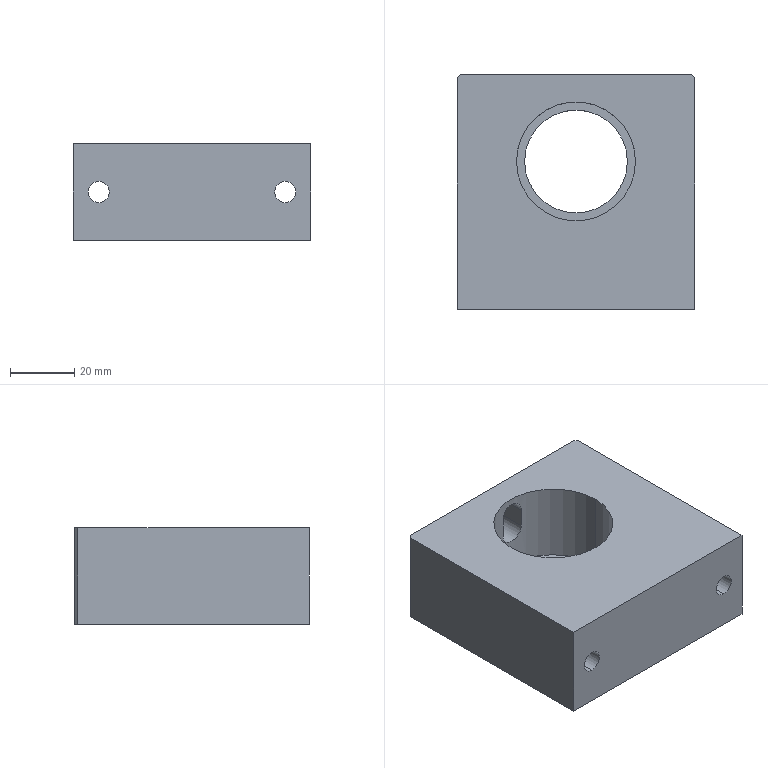Part | SolidWorks | features BaseBody 1 | 1 solid | 28 faces | box 74 x 73 x 30 mm | volume 117987 mm3 | cylinder 15 | plane 13 | commonest cylinder face diameters 6.6 x4 11 x4 8 x3 32 x2 37 x2
STEP:
#1=CARTESIAN_POINT('',(0.,28.,28.));
#2=VERTEX_POINT('',#1);
#3=CARTESIAN_POINT('',(4.,27.562,24.));
#4=VERTEX_POINT('',#3);
#5=CARTESIAN_POINT('',(0.,28.,28.));
#6=CARTESIAN_POINT('',(0.265,28.,28.));
#7=CARTESIAN_POINT('',(0.5253,27.994,27.974));
#8=CARTESIAN_POINT('',(1.037,27.973,27.872));
#9=CARTESIAN_POINT('',(1.292,27.956,27.795));
#10=CARTESIAN_POINT('',(1.776,27.916,27.594));
#11=CARTESIAN_POINT('',(2.005,27.892,27.471));
#12=CARTESIAN_POINT('',(2.439,27.84,27.181));
#13=CARTESIAN_POINT('',(2.644,27.811,27.013));
#14=CARTESIAN_POINT('',(3.012,27.754,26.645));
#15=CARTESIAN_POINT('',(3.177,27.726,26.445));
#16=CARTESIAN_POINT('',(3.469,27.672,26.008));
#17=CARTESIAN_POINT('',(3.593,27.648,25.777));
#18=CARTESIAN_POINT('',(3.793,27.607,25.296));
#19=CARTESIAN_POINT('',(3.87,27.591,25.044));
#20=CARTESIAN_POINT('',(3.974,27.568,24.527));
#21=CARTESIAN_POINT('',(4.,27.562,24.265));
#22=CARTESIAN_POINT('',(4.,27.562,24.));
#23=B_SPLINE_CURVE_WITH_KNOTS('',3,(#5,#6,#7,#8,#9,#10,#11,#12,#13,#14,#15,#16,#17,#18,#19,#20,#21,#22),.UNSPECIFIED.,.F.,.F.,(4,2,2,2,2,2,2,2,4),(0.,0.0007834,0.001567,0.00235,0.003134,0.003917,0.0047,0.005484,0.006267),.UNSPECIFIED.);
#24=EDGE_CURVE('',#2,#4,#23,.T.);
#25=ORIENTED_EDGE('',*,*,#24,.F.);
#26=CARTESIAN_POINT('',(0.,36.5,28.));
#27=VERTEX_POINT('',#26);
#28=CARTESIAN_POINT('',(0.,11.5,28.));
#29=DIRECTION('',(0.,1.,0.));
#30=VECTOR('',#29,1000.);
#31=LINE('',#28,#30);
#32=EDGE_CURVE('',#2,#27,#31,.T.);
#33=ORIENTED_EDGE('',*,*,#32,.T.);
#34=CARTESIAN_POINT('',(4.,36.5,24.));
#35=VERTEX_POINT('',#34);
#36=CARTESIAN_POINT('',(0.,36.5,24.));
#37=DIRECTION('',(0.,1.,0.));
#38=DIRECTION('',(0.,0.,1.));
#39=AXIS2_PLACEMENT_3D('',#36,#37,#38);
#40=CIRCLE('',#39,4.);
#41=EDGE_CURVE('',#27,#35,#40,.T.);
#42=ORIENTED_EDGE('',*,*,#41,.T.);
#43=CARTESIAN_POINT('',(4.,11.5,24.));
#44=DIRECTION('',(0.,1.,0.));
#45=VECTOR('',#44,1000.);
#46=LINE('',#43,#45);
#47=EDGE_CURVE('',#4,#35,#46,.T.);
#48=ORIENTED_EDGE('',*,*,#47,.F.);
#49=EDGE_LOOP('',(#25,#33,#42,#48));
#50=FACE_OUTER_BOUND('',#49,.T.);
#51=CARTESIAN_POINT('',(0.,11.5,24.));
#52=DIRECTION('',(0.,1.,0.));
#53=DIRECTION('',(0.,0.,1.));
#54=AXIS2_PLACEMENT_3D('',#51,#52,#53);
#55=CYLINDRICAL_SURFACE('',#54,4.);
#56=ADVANCED_FACE('',(#50),#55,.F.);
#57=CARTESIAN_POINT('',(-29.,-23.5,9.5));
#58=VERTEX_POINT('',#57);
#59=CARTESIAN_POINT('',(-29.,-23.5,20.5));
#60=VERTEX_POINT('',#59);
#61=CARTESIAN_POINT('',(-29.,-23.5,15.));
#62=DIRECTION('',(0.,1.,0.));
#63=DIRECTION('',(0.,0.,1.));
#64=AXIS2_PLACEMENT_3D('',#61,#62,#63);
#65=CIRCLE('',#64,5.5);
#66=EDGE_CURVE('',#58,#60,#65,.T.);
#67=ORIENTED_EDGE('',*,*,#66,.F.);
#68=CARTESIAN_POINT('',(-29.,36.5,9.5));
#69=VERTEX_POINT('',#68);
#70=CARTESIAN_POINT('',(-29.,36.5,9.5));
#71=DIRECTION('',(0.,1.,0.));
#72=VECTOR('',#71,1000.);
#73=LINE('',#70,#72);
#74=EDGE_CURVE('',#58,#69,#73,.T.);
#75=ORIENTED_EDGE('',*,*,#74,.T.);
#76=CARTESIAN_POINT('',(-29.,36.5,20.5));
#77=VERTEX_POINT('',#76);
#78=CARTESIAN_POINT('',(-29.,36.5,15.));
#79=DIRECTION('',(0.,1.,0.));
#80=DIRECTION('',(0.,0.,1.));
#81=AXIS2_PLACEMENT_3D('',#78,#79,#80);
#82=CIRCLE('',#81,5.5);
#83=EDGE_CURVE('',#69,#77,#82,.T.);
#84=ORIENTED_EDGE('',*,*,#83,.T.);
#85=CARTESIAN_POINT('',(-29.,36.5,20.5));
#86=DIRECTION('',(0.,1.,0.));
#87=VECTOR('',#86,1000.);
#88=LINE('',#85,#87);
#89=EDGE_CURVE('',#60,#77,#88,.T.);
#90=ORIENTED_EDGE('',*,*,#89,.F.);
#91=EDGE_LOOP('',(#67,#75,#84,#90));
#92=FACE_OUTER_BOUND('',#91,.T.);
#93=CARTESIAN_POINT('',(-29.,36.5,15.));
#94=DIRECTION('',(0.,1.,0.));
#95=DIRECTION('',(0.,0.,1.));
#96=AXIS2_PLACEMENT_3D('',#93,#94,#95);
#97=CYLINDRICAL_SURFACE('',#96,5.5);
#98=ADVANCED_FACE('',(#92),#97,.F.);
#99=CARTESIAN_POINT('',(-29.,-36.5,11.7));
#100=VERTEX_POINT('',#99);
#101=CARTESIAN_POINT('',(-29.,-36.5,18.3));
#102=VERTEX_POINT('',#101);
#103=CARTESIAN_POINT('',(-29.,-36.5,15.));
#104=DIRECTION('',(0.,1.,0.));
#105=DIRECTION('',(0.,0.,1.));
#106=AXIS2_PLACEMENT_3D('',#103,#104,#105);
#107=CIRCLE('',#106,3.3);
#108=EDGE_CURVE('',#100,#102,#107,.T.);
#109=ORIENTED_EDGE('',*,*,#108,.F.);
#110=CARTESIAN_POINT('',(-29.,-23.5,11.7));
#111=VERTEX_POINT('',#110);
#112=CARTESIAN_POINT('',(-29.,36.5,11.7));
#113=DIRECTION('',(0.,1.,0.));
#114=VECTOR('',#113,1000.);
#115=LINE('',#112,#114);
#116=EDGE_CURVE('',#100,#111,#115,.T.);
#117=ORIENTED_EDGE('',*,*,#116,.T.);
#118=CARTESIAN_POINT('',(-29.,-23.5,18.3));
#119=VERTEX_POINT('',#118);
#120=CARTESIAN_POINT('',(-29.,-23.5,15.));
#121=DIRECTION('',(0.,1.,0.));
#122=DIRECTION('',(0.,0.,1.));
#123=AXIS2_PLACEMENT_3D('',#120,#121,#122);
#124=CIRCLE('',#123,3.3);
#125=EDGE_CURVE('',#111,#119,#124,.T.);
#126=ORIENTED_EDGE('',*,*,#125,.T.);
#127=CARTESIAN_POINT('',(-29.,36.5,18.3));
#128=DIRECTION('',(0.,1.,0.));
#129=VECTOR('',#128,1000.);
#130=LINE('',#127,#129);
#131=EDGE_CURVE('',#102,#119,#130,.T.);
#132=ORIENTED_EDGE('',*,*,#131,.F.);
#133=EDGE_LOOP('',(#109,#117,#126,#132));
#134=FACE_OUTER_BOUND('',#133,.T.);
#135=CARTESIAN_POINT('',(-29.,36.5,15.));
#136=DIRECTION('',(0.,1.,0.));
#137=DIRECTION('',(0.,0.,1.));
#138=AXIS2_PLACEMENT_3D('',#135,#136,#137);
#139=CYLINDRICAL_SURFACE('',#138,3.3);
#140=ADVANCED_FACE('',(#134),#139,.F.);
#141=CARTESIAN_POINT('',(29.,-23.5,9.5));
#142=VERTEX_POINT('',#141);
#143=CARTESIAN_POINT('',(29.,-23.5,20.5));
#144=VERTEX_POINT('',#143);
#145=CARTESIAN_POINT('',(29.,-23.5,15.));
#146=DIRECTION('',(0.,1.,0.));
#147=DIRECTION('',(0.,0.,1.));
#148=AXIS2_PLACEMENT_3D('',#145,#146,#147);
#149=CIRCLE('',#148,5.5);
#150=EDGE_CURVE('',#142,#144,#149,.T.);
#151=ORIENTED_EDGE('',*,*,#150,.F.);
#152=CARTESIAN_POINT('',(29.,36.5,9.5));
#153=VERTEX_POINT('',#152);
#154=CARTESIAN_POINT('',(29.,36.5,9.5));
#155=DIRECTION('',(0.,1.,0.));
#156=VECTOR('',#155,1000.);
#157=LINE('',#154,#156);
#158=EDGE_CURVE('',#142,#153,#157,.T.);
#159=ORIENTED_EDGE('',*,*,#158,.T.);
#160=CARTESIAN_POINT('',(29.,36.5,20.5));
#161=VERTEX_POINT('',#160);
#162=CARTESIAN_POINT('',(29.,36.5,15.));
#163=DIRECTION('',(0.,1.,0.));
#164=DIRECTION('',(0.,0.,1.));
#165=AXIS2_PLACEMENT_3D('',#162,#163,#164);
#166=CIRCLE('',#165,5.5);
#167=EDGE_CURVE('',#153,#161,#166,.T.);
#168=ORIENTED_EDGE('',*,*,#167,.T.);
#169=CARTESIAN_POINT('',(29.,36.5,20.5));
#170=DIRECTION('',(0.,1.,0.));
#171=VECTOR('',#170,1000.);
#172=LINE('',#169,#171);
#173=EDGE_CURVE('',#144,#161,#172,.T.);
#174=ORIENTED_EDGE('',*,*,#173,.F.);
#175=EDGE_LOOP('',(#151,#159,#168,#174));
#176=FACE_OUTER_BOUND('',#175,.T.);
#177=CARTESIAN_POINT('',(29.,36.5,15.));
#178=DIRECTION('',(0.,1.,0.));
#179=DIRECTION('',(0.,0.,1.));
#180=AXIS2_PLACEMENT_3D('',#177,#178,#179);
#181=CYLINDRICAL_SURFACE('',#180,5.5);
#182=ADVANCED_FACE('',(#176),#181,.F.);
#183=CARTESIAN_POINT('',(29.,-36.5,11.7));
#184=VERTEX_POINT('',#183);
#185=CARTESIAN_POINT('',(29.,-36.5,18.3));
#186=VERTEX_POINT('',#185);
#187=CARTESIAN_POINT('',(29.,-36.5,15.));
#188=DIRECTION('',(0.,1.,0.));
#189=DIRECTION('',(0.,0.,1.));
#190=AXIS2_PLACEMENT_3D('',#187,#188,#189);
#191=CIRCLE('',#190,3.3);
#192=EDGE_CURVE('',#184,#186,#191,.T.);
#193=ORIENTED_EDGE('',*,*,#192,.F.);
#194=CARTESIAN_POINT('',(29.,-23.5,11.7));
#195=VERTEX_POINT('',#194);
#196=CARTESIAN_POINT('',(29.,36.5,11.7));
#197=DIRECTION('',(0.,1.,0.));
#198=VECTOR('',#197,1000.);
#199=LINE('',#196,#198);
#200=EDGE_CURVE('',#184,#195,#199,.T.);
#201=ORIENTED_EDGE('',*,*,#200,.T.);
#202=CARTESIAN_POINT('',(29.,-23.5,18.3));
#203=VERTEX_POINT('',#202);
#204=CARTESIAN_POINT('',(29.,-23.5,15.));
#205=DIRECTION('',(0.,1.,0.));
#206=DIRECTION('',(0.,0.,1.));
#207=AXIS2_PLACEMENT_3D('',#204,#205,#206);
#208=CIRCLE('',#207,3.3);
#209=EDGE_CURVE('',#195,#203,#208,.T.);
#210=ORIENTED_EDGE('',*,*,#209,.T.);
#211=CARTESIAN_POINT('',(29.,36.5,18.3));
#212=DIRECTION('',(0.,1.,0.));
#213=VECTOR('',#212,1000.);
#214=LINE('',#211,#213);
#215=EDGE_CURVE('',#186,#203,#214,.T.);
#216=ORIENTED_EDGE('',*,*,#215,.F.);
#217=EDGE_LOOP('',(#193,#201,#210,#216));
#218=FACE_OUTER_BOUND('',#217,.T.);
#219=CARTESIAN_POINT('',(29.,36.5,15.));
#220=DIRECTION('',(0.,1.,0.));
#221=DIRECTION('',(0.,0.,1.));
#222=AXIS2_PLACEMENT_3D('',#219,#220,#221);
#223=CYLINDRICAL_SURFACE('',#222,3.3);
#224=ADVANCED_FACE('',(#218),#223,.F.);
#225=CARTESIAN_POINT('',(-18.5,9.5,5.));
#226=VERTEX_POINT('',#225);
#227=CARTESIAN_POINT('',(18.5,9.5,5.));
#228=VERTEX_POINT('',#227);
#229=CARTESIAN_POINT('',(0.,9.5,5.));
#230=DIRECTION('',(0.,0.,1.));
#231=DIRECTION('',(1.,0.,0.));
#232=AXIS2_PLACEMENT_3D('',#229,#230,#231);
#233=CIRCLE('',#232,18.5);
#234=EDGE_CURVE('',#226,#228,#233,.T.);
#235=ORIENTED_EDGE('',*,*,#234,.F.);
#236=CARTESIAN_POINT('',(-18.5,9.5,30.));
#237=VERTEX_POINT('',#236);
#238=CARTESIAN_POINT('',(-18.5,9.5,5.));
#239=DIRECTION('',(0.,0.,1.));
#240=VECTOR('',#239,1000.);
#241=LINE('',#238,#240);
#242=EDGE_CURVE('',#226,#237,#241,.T.);
#243=ORIENTED_EDGE('',*,*,#242,.T.);
#244=CARTESIAN_POINT('',(18.5,9.5,30.));
#245=VERTEX_POINT('',#244);
#246=CARTESIAN_POINT('',(0.,9.5,30.));
#247=DIRECTION('',(0.,0.,1.));
#248=DIRECTION('',(1.,0.,0.));
#249=AXIS2_PLACEMENT_3D('',#246,#247,#248);
#250=CIRCLE('',#249,18.5);
#251=EDGE_CURVE('',#237,#245,#250,.T.);
#252=ORIENTED_EDGE('',*,*,#251,.T.);
#253=CARTESIAN_POINT('',(18.5,9.5,5.));
#254=DIRECTION('',(0.,0.,1.));
#255=VECTOR('',#254,1000.);
#256=LINE('',#253,#255);
#257=EDGE_CURVE('',#228,#245,#256,.T.);
#258=ORIENTED_EDGE('',*,*,#257,.F.);
#259=EDGE_LOOP('',(#235,#243,#252,#258));
#260=FACE_OUTER_BOUND('',#259,.T.);
#261=CARTESIAN_POINT('',(0.,9.5,5.));
#262=DIRECTION('',(0.,0.,1.));
#263=DIRECTION('',(1.,0.,0.));
#264=AXIS2_PLACEMENT_3D('',#261,#262,#263);
#265=CYLINDRICAL_SURFACE('',#264,18.5);
#266=ADVANCED_FACE('',(#260),#265,.F.);
#267=CARTESIAN_POINT('',(-16.,9.5,0.));
#268=VERTEX_POINT('',#267);
#269=CARTESIAN_POINT('',(16.,9.5,0.));
#270=VERTEX_POINT('',#269);
#271=CARTESIAN_POINT('',(0.,9.5,0.));
#272=DIRECTION('',(0.,0.,1.));
#273=DIRECTION('',(1.,0.,0.));
#274=AXIS2_PLACEMENT_3D('',#271,#272,#273);
#275=CIRCLE('',#274,16.);
#276=EDGE_CURVE('',#268,#270,#275,.T.);
#277=ORIENTED_EDGE('',*,*,#276,.F.);
#278=CARTESIAN_POINT('',(-16.,9.5,5.));
#279=VERTEX_POINT('',#278);
#280=CARTESIAN_POINT('',(-16.,9.5,0.));
#281=DIRECTION('',(0.,0.,1.));
#282=VECTOR('',#281,1000.);
#283=LINE('',#280,#282);
#284=EDGE_CURVE('',#268,#279,#283,.T.);
#285=ORIENTED_EDGE('',*,*,#284,.T.);
#286=CARTESIAN_POINT('',(16.,9.5,5.));
#287=VERTEX_POINT('',#286);
#288=CARTESIAN_POINT('',(0.,9.5,5.));
#289=DIRECTION('',(0.,0.,-1.));
#290=DIRECTION('',(1.,0.,0.));
#291=AXIS2_PLACEMENT_3D('',#288,#289,#290);
#292=CIRCLE('',#291,16.);
#293=EDGE_CURVE('',#287,#279,#292,.T.);
#294=ORIENTED_EDGE('',*,*,#293,.F.);
#295=CARTESIAN_POINT('',(16.,9.5,0.));
#296=DIRECTION('',(0.,0.,1.));
#297=VECTOR('',#296,1000.);
#298=LINE('',#295,#297);
#299=EDGE_CURVE('',#270,#287,#298,.T.);
#300=ORIENTED_EDGE('',*,*,#299,.F.);
#301=EDGE_LOOP('',(#277,#285,#294,#300));
#302=FACE_OUTER_BOUND('',#301,.T.);
#303=CARTESIAN_POINT('',(0.,9.5,0.));
#304=DIRECTION('',(0.,0.,1.));
#305=DIRECTION('',(1.,0.,0.));
#306=AXIS2_PLACEMENT_3D('',#303,#304,#305);
#307=CYLINDRICAL_SURFACE('',#306,16.);
#308=ADVANCED_FACE('',(#302),#307,.F.);
#309=CARTESIAN_POINT('',(37.,35.5,30.));
#310=VERTEX_POINT('',#309);
#311=CARTESIAN_POINT('',(36.,36.5,30.));
#312=VERTEX_POINT('',#311);
#313=CARTESIAN_POINT('',(36.25,36.25,30.));
#314=DIRECTION('',(-0.7071,0.7071,0.));
#315=VECTOR('',#314,1000.);
#316=LINE('',#313,#315);
#317=EDGE_CURVE('',#310,#312,#316,.T.);
#318=ORIENTED_EDGE('',*,*,#317,.F.);
#319=CARTESIAN_POINT('',(37.,35.5,0.));
#320=VERTEX_POINT('',#319);
#321=CARTESIAN_POINT('',(37.,35.5,30.));
#322=DIRECTION('',(0.,0.,1.));
#323=VECTOR('',#322,1000.);
#324=LINE('',#321,#323);
#325=EDGE_CURVE('',#320,#310,#324,.T.);
#326=ORIENTED_EDGE('',*,*,#325,.F.);
#327=CARTESIAN_POINT('',(36.,36.5,0.));
#328=VERTEX_POINT('',#327);
#329=CARTESIAN_POINT('',(36.,36.5,0.));
#330=DIRECTION('',(0.7071,-0.7071,0.));
#331=VECTOR('',#330,1000.);
#332=LINE('',#329,#331);
#333=EDGE_CURVE('',#328,#320,#332,.T.);
#334=ORIENTED_EDGE('',*,*,#333,.F.);
#335=CARTESIAN_POINT('',(36.,36.5,30.));
#336=DIRECTION('',(0.,0.,-1.));
#337=VECTOR('',#336,1000.);
#338=LINE('',#335,#337);
#339=EDGE_CURVE('',#312,#328,#338,.T.);
#340=ORIENTED_EDGE('',*,*,#339,.F.);
#341=EDGE_LOOP('',(#318,#326,#334,#340));
#342=FACE_OUTER_BOUND('',#341,.T.);
#343=CARTESIAN_POINT('',(36.,36.5,30.));
#344=DIRECTION('',(-0.7071,-0.7071,0.));
#345=DIRECTION('',(-0.7071,0.7071,0.));
#346=AXIS2_PLACEMENT_3D('',#343,#344,#345);
#347=PLANE('',#346);
#348=ADVANCED_FACE('',(#342),#347,.F.);
#349=CARTESIAN_POINT('',(-36.,36.5,30.));
#350=VERTEX_POINT('',#349);
#351=CARTESIAN_POINT('',(-37.,35.5,30.));
#352=VERTEX_POINT('',#351);
#353=CARTESIAN_POINT('',(-36.25,36.25,30.));
#354=DIRECTION('',(-0.7071,-0.7071,0.));
#355=VECTOR('',#354,1000.);
#356=LINE('',#353,#355);
#357=EDGE_CURVE('',#350,#352,#356,.T.);
#358=ORIENTED_EDGE('',*,*,#357,.F.);
#359=CARTESIAN_POINT('',(-36.,36.5,0.));
#360=VERTEX_POINT('',#359);
#361=CARTESIAN_POINT('',(-36.,36.5,30.));
#362=DIRECTION('',(0.,0.,1.));
#363=VECTOR('',#362,1000.);
#364=LINE('',#361,#363);
#365=EDGE_CURVE('',#360,#350,#364,.T.);
#366=ORIENTED_EDGE('',*,*,#365,.F.);
#367=CARTESIAN_POINT('',(-37.,35.5,0.));
#368=VERTEX_POINT('',#367);
#369=CARTESIAN_POINT('',(-37.,35.5,0.));
#370=DIRECTION('',(0.7071,0.7071,0.));
#371=VECTOR('',#370,1000.);
#372=LINE('',#369,#371);
#373=EDGE_CURVE('',#368,#360,#372,.T.);
#374=ORIENTED_EDGE('',*,*,#373,.F.);
#375=CARTESIAN_POINT('',(-37.,35.5,30.));
#376=DIRECTION('',(0.,0.,-1.));
#377=VECTOR('',#376,1000.);
#378=LINE('',#375,#377);
#379=EDGE_CURVE('',#352,#368,#378,.T.);
#380=ORIENTED_EDGE('',*,*,#379,.F.);
#381=EDGE_LOOP('',(#358,#366,#374,#380));
#382=FACE_OUTER_BOUND('',#381,.T.);
#383=CARTESIAN_POINT('',(-37.,35.5,30.));
#384=DIRECTION('',(0.7071,-0.7071,0.));
#385=DIRECTION('',(0.,0.,-1.));
#386=AXIS2_PLACEMENT_3D('',#383,#384,#385);
#387=PLANE('',#386);
#388=ADVANCED_FACE('',(#382),#387,.F.);
#389=CARTESIAN_POINT('',(-4.,27.562,18.));
#390=VERTEX_POINT('',#389);
#391=CARTESIAN_POINT('',(-4.,36.5,18.));
#392=VERTEX_POINT('',#391);
#393=CARTESIAN_POINT('',(-4.,11.5,18.));
#394=DIRECTION('',(0.,1.,0.));
#395=VECTOR('',#394,1000.);
#396=LINE('',#393,#395);
#397=EDGE_CURVE('',#390,#392,#396,.T.);
#398=ORIENTED_EDGE('',*,*,#397,.T.);
#399=CARTESIAN_POINT('',(-4.,36.5,24.));
#400=VERTEX_POINT('',#399);
#401=CARTESIAN_POINT('',(-4.,36.5,18.));
#402=DIRECTION('',(0.,0.,1.));
#403=VECTOR('',#402,1000.);
#404=LINE('',#401,#403);
#405=EDGE_CURVE('',#392,#400,#404,.T.);
#406=ORIENTED_EDGE('',*,*,#405,.T.);
#407=CARTESIAN_POINT('',(-4.,27.562,24.));
#408=VERTEX_POINT('',#407);
#409=CARTESIAN_POINT('',(-4.,11.5,24.));
#410=DIRECTION('',(0.,1.,0.));
#411=VECTOR('',#410,1000.);
#412=LINE('',#409,#411);
#413=EDGE_CURVE('',#408,#400,#412,.T.);
#414=ORIENTED_EDGE('',*,*,#413,.F.);
#415=CARTESIAN_POINT('',(-4.,27.562,5.));
#416=DIRECTION('',(0.,0.,1.));
#417=VECTOR('',#416,1000.);
#418=LINE('',#415,#417);
#419=EDGE_CURVE('',#390,#408,#418,.T.);
#420=ORIENTED_EDGE('',*,*,#419,.F.);
#421=EDGE_LOOP('',(#398,#406,#414,#420));
#422=FACE_OUTER_BOUND('',#421,.T.);
#423=CARTESIAN_POINT('',(-4.,11.5,18.));
#424=DIRECTION('',(-1.,0.,0.));
#425=DIRECTION('',(0.,1.,0.));
#426=AXIS2_PLACEMENT_3D('',#423,#424,#425);
#427=PLANE('',#426);
#428=ADVANCED_FACE('',(#422),#427,.F.);
#429=ORIENTED_EDGE('',*,*,#47,.T.);
#430=CARTESIAN_POINT('',(4.,36.5,18.));
#431=VERTEX_POINT('',#430);
#432=CARTESIAN_POINT('',(4.,36.5,18.));
#433=DIRECTION('',(0.,0.,-1.));
#434=VECTOR('',#433,1000.);
#435=LINE('',#432,#434);
#436=EDGE_CURVE('',#35,#431,#435,.T.);
#437=ORIENTED_EDGE('',*,*,#436,.T.);
#438=CARTESIAN_POINT('',(4.,27.562,18.));
#439=VERTEX_POINT('',#438);
#440=CARTESIAN_POINT('',(4.,11.5,18.));
#441=DIRECTION('',(0.,1.,0.));
#442=VECTOR('',#441,1000.);
#443=LINE('',#440,#442);
#444=EDGE_CURVE('',#439,#431,#443,.T.);
#445=ORIENTED_EDGE('',*,*,#444,.F.);
#446=CARTESIAN_POINT('',(4.,27.562,5.));
#447=DIRECTION('',(0.,0.,-1.));
#448=VECTOR('',#447,1000.);
#449=LINE('',#446,#448);
#450=EDGE_CURVE('',#4,#439,#449,.T.);
#451=ORIENTED_EDGE('',*,*,#450,.F.);
#452=EDGE_LOOP('',(#429,#437,#445,#451));
#453=FACE_OUTER_BOUND('',#452,.T.);
#454=CARTESIAN_POINT('',(4.,11.5,18.));
#455=DIRECTION('',(1.,0.,0.));
#456=DIRECTION('',(0.,1.,0.));
#457=AXIS2_PLACEMENT_3D('',#454,#455,#456);
#458=PLANE('',#457);
#459=ADVANCED_FACE('',(#453),#458,.F.);
#460=ORIENTED_EDGE('',*,*,#444,.T.);
#461=CARTESIAN_POINT('',(0.,36.5,18.));
#462=DIRECTION('',(0.,1.,0.));
#463=DIRECTION('',(0.,0.,1.));
#464=AXIS2_PLACEMENT_3D('',#461,#462,#463);
#465=CIRCLE('',#464,4.);
#466=EDGE_CURVE('',#431,#392,#465,.T.);
#467=ORIENTED_EDGE('',*,*,#466,.T.);
#468=ORIENTED_EDGE('',*,*,#397,.F.);
#469=CARTESIAN_POINT('',(4.,27.562,18.));
#470=CARTESIAN_POINT('',(4.,27.562,17.735));
#471=CARTESIAN_POINT('',(3.974,27.568,17.474));
#472=CARTESIAN_POINT('',(3.872,27.59,16.962));
#473=CARTESIAN_POINT('',(3.795,27.607,16.708));
#474=CARTESIAN_POINT('',(3.594,27.648,16.224));
#475=CARTESIAN_POINT('',(3.471,27.672,15.995));
#476=CARTESIAN_POINT('',(3.181,27.725,15.56));
#477=CARTESIAN_POINT('',(3.012,27.754,15.355));
#478=CARTESIAN_POINT('',(2.645,27.811,14.988));
#479=CARTESIAN_POINT('',(2.444,27.839,14.822));
#480=CARTESIAN_POINT('',(2.007,27.892,14.53));
#481=CARTESIAN_POINT('',(1.775,27.916,14.406));
#482=CARTESIAN_POINT('',(1.295,27.956,14.206));
#483=CARTESIAN_POINT('',(1.042,27.972,14.129));
#484=CARTESIAN_POINT('',(0.525,27.994,14.026));
#485=CARTESIAN_POINT('',(0.265,28.,14.));
#486=CARTESIAN_POINT('',(-0.2584,28.,14.));
#487=CARTESIAN_POINT('',(-0.5243,27.994,14.026));
#488=CARTESIAN_POINT('',(-1.038,27.973,14.128));
#489=CARTESIAN_POINT('',(-1.288,27.957,14.204));
#490=CARTESIAN_POINT('',(-1.773,27.916,14.405));
#491=CARTESIAN_POINT('',(-2.006,27.892,14.53));
#492=CARTESIAN_POINT('',(-2.438,27.84,14.818));
#493=CARTESIAN_POINT('',(-2.641,27.811,14.985));
#494=CARTESIAN_POINT('',(-3.013,27.754,15.356));
#495=CARTESIAN_POINT('',(-3.178,27.726,15.557));
#496=CARTESIAN_POINT('',(-3.468,27.673,15.989));
#497=CARTESIAN_POINT('',(-3.593,27.648,16.223));
#498=CARTESIAN_POINT('',(-3.794,27.607,16.706));
#499=CARTESIAN_POINT('',(-3.87,27.591,16.955));
#500=CARTESIAN_POINT('',(-3.973,27.568,17.47));
#501=CARTESIAN_POINT('',(-4.,27.562,17.735));
#502=CARTESIAN_POINT('',(-4.,27.562,18.));
#503=B_SPLINE_CURVE_WITH_KNOTS('',3,(#469,#470,#471,#472,#473,#474,#475,#476,#477,#478,#479,#480,#481,#482,#483,#484,#485,#486,#487,#488,#489,#490,#491,#492,#493,#494,#495,#496,#497,#498,#499,#500,#501,#502),.UNSPECIFIED.,.F.,.F.,(4,2,2,2,2,2,2,2,2,2,2,2,2,2,2,2,4),(0.,0.0007837,0.001567,0.002351,0.003135,0.003919,0.004702,0.005486,0.00627,0.007053,0.007837,0.008621,0.009405,0.01019,0.01097,0.01176,0.01254),.UNSPECIFIED.);
#504=EDGE_CURVE('',#439,#390,#503,.T.);
#505=ORIENTED_EDGE('',*,*,#504,.F.);
#506=EDGE_LOOP('',(#460,#467,#468,#505));
#507=FACE_OUTER_BOUND('',#506,.T.);
#508=CARTESIAN_POINT('',(0.,11.5,18.));
#509=DIRECTION('',(0.,1.,0.));
#510=DIRECTION('',(0.,0.,1.));
#511=AXIS2_PLACEMENT_3D('',#508,#509,#510);
#512=CYLINDRICAL_SURFACE('',#511,4.);
#513=ADVANCED_FACE('',(#507),#512,.F.);
#514=CARTESIAN_POINT('',(-29.,-23.5,15.));
#515=DIRECTION('',(0.,1.,0.));
#516=DIRECTION('',(0.,0.,1.));
#517=AXIS2_PLACEMENT_3D('',#514,#515,#516);
#518=CIRCLE('',#517,3.3);
#519=EDGE_CURVE('',#119,#111,#518,.T.);
#520=ORIENTED_EDGE('',*,*,#519,.F.);
#521=ORIENTED_EDGE('',*,*,#125,.F.);
#522=EDGE_LOOP('',(#520,#521));
#523=FACE_BOUND('',#522,.T.);
#524=CARTESIAN_POINT('',(-29.,-23.5,15.));
#525=DIRECTION('',(0.,1.,0.));
#526=DIRECTION('',(0.,0.,1.));
#527=AXIS2_PLACEMENT_3D('',#524,#525,#526);
#528=CIRCLE('',#527,5.5);
#529=EDGE_CURVE('',#60,#58,#528,.T.);
#530=ORIENTED_EDGE('',*,*,#529,.T.);
#531=ORIENTED_EDGE('',*,*,#66,.T.);
#532=EDGE_LOOP('',(#530,#531));
#533=FACE_OUTER_BOUND('',#532,.T.);
#534=CARTESIAN_POINT('',(-25.7,-23.5,15.));
#535=DIRECTION('',(0.,-1.,0.));
#536=DIRECTION('',(0.,0.,-1.));
#537=AXIS2_PLACEMENT_3D('',#534,#535,#536);
#538=PLANE('',#537);
#539=ADVANCED_FACE('',(#523,#533),#538,.F.);
#540=CARTESIAN_POINT('',(29.,-23.5,15.));
#541=DIRECTION('',(0.,1.,0.));
#542=DIRECTION('',(0.,0.,1.));
#543=AXIS2_PLACEMENT_3D('',#540,#541,#542);
#544=CIRCLE('',#543,3.3);
#545=EDGE_CURVE('',#203,#195,#544,.T.);
#546=ORIENTED_EDGE('',*,*,#545,.F.);
#547=ORIENTED_EDGE('',*,*,#209,.F.);
#548=EDGE_LOOP('',(#546,#547));
#549=FACE_BOUND('',#548,.T.);
#550=CARTESIAN_POINT('',(29.,-23.5,15.));
#551=DIRECTION('',(0.,1.,0.));
#552=DIRECTION('',(0.,0.,1.));
#553=AXIS2_PLACEMENT_3D('',#550,#551,#552);
#554=CIRCLE('',#553,5.5);
#555=EDGE_CURVE('',#144,#142,#554,.T.);
#556=ORIENTED_EDGE('',*,*,#555,.T.);
#557=ORIENTED_EDGE('',*,*,#150,.T.);
#558=EDGE_LOOP('',(#556,#557));
#559=FACE_OUTER_BOUND('',#558,.T.);
#560=CARTESIAN_POINT('',(32.3,-23.5,15.));
#561=DIRECTION('',(0.,-1.,0.));
#562=DIRECTION('',(0.,0.,-1.));
#563=AXIS2_PLACEMENT_3D('',#560,#561,#562);
#564=PLANE('',#563);
#565=ADVANCED_FACE('',(#549,#559),#564,.F.);
#566=ORIENTED_EDGE('',*,*,#293,.T.);
#567=CARTESIAN_POINT('',(0.,9.5,5.));
#568=DIRECTION('',(0.,0.,-1.));
#569=DIRECTION('',(1.,0.,0.));
#570=AXIS2_PLACEMENT_3D('',#567,#568,#569);
#571=CIRCLE('',#570,16.);
#572=EDGE_CURVE('',#279,#287,#571,.T.);
#573=ORIENTED_EDGE('',*,*,#572,.T.);
#574=EDGE_LOOP('',(#566,#573));
#575=FACE_BOUND('',#574,.T.);
#576=CARTESIAN_POINT('',(0.,9.5,5.));
#577=DIRECTION('',(0.,0.,1.));
#578=DIRECTION('',(1.,0.,0.));
#579=AXIS2_PLACEMENT_3D('',#576,#577,#578);
#580=CIRCLE('',#579,18.5);
#581=EDGE_CURVE('',#228,#226,#580,.T.);
#582=ORIENTED_EDGE('',*,*,#581,.T.);
#583=ORIENTED_EDGE('',*,*,#234,.T.);
#584=EDGE_LOOP('',(#582,#583));
#585=FACE_OUTER_BOUND('',#584,.T.);
#586=CARTESIAN_POINT('',(0.,9.5,5.));
#587=DIRECTION('',(0.,0.,1.));
#588=DIRECTION('',(1.,0.,0.));
#589=AXIS2_PLACEMENT_3D('',#586,#587,#588);
#590=PLANE('',#589);
#591=ADVANCED_FACE('',(#575,#585),#590,.T.);
#592=CARTESIAN_POINT('',(0.,9.5,0.));
#593=DIRECTION('',(0.,0.,1.));
#594=DIRECTION('',(1.,0.,0.));
#595=AXIS2_PLACEMENT_3D('',#592,#593,#594);
#596=CIRCLE('',#595,16.);
#597=EDGE_CURVE('',#270,#268,#596,.T.);
#598=ORIENTED_EDGE('',*,*,#597,.T.);
#599=ORIENTED_EDGE('',*,*,#276,.T.);
#600=EDGE_LOOP('',(#598,#599));
#601=FACE_BOUND('',#600,.T.);
#602=CARTESIAN_POINT('',(-37.,-36.5,0.));
#603=VERTEX_POINT('',#602);
#604=CARTESIAN_POINT('',(-37.,36.5,0.));
#605=DIRECTION('',(0.,-1.,0.));
#606=VECTOR('',#605,1000.);
#607=LINE('',#604,#606);
#608=EDGE_CURVE('',#368,#603,#607,.T.);
#609=ORIENTED_EDGE('',*,*,#608,.F.);
#610=ORIENTED_EDGE('',*,*,#373,.T.);
#611=CARTESIAN_POINT('',(-37.,36.5,0.));
#612=DIRECTION('',(-1.,0.,0.));
#613=VECTOR('',#612,1000.);
#614=LINE('',#611,#613);
#615=EDGE_CURVE('',#328,#360,#614,.T.);
#616=ORIENTED_EDGE('',*,*,#615,.F.);
#617=ORIENTED_EDGE('',*,*,#333,.T.);
#618=CARTESIAN_POINT('',(37.,-36.5,0.));
#619=VERTEX_POINT('',#618);
#620=CARTESIAN_POINT('',(37.,36.5,0.));
#621=DIRECTION('',(0.,1.,0.));
#622=VECTOR('',#621,1000.);
#623=LINE('',#620,#622);
#624=EDGE_CURVE('',#619,#320,#623,.T.);
#625=ORIENTED_EDGE('',*,*,#624,.F.);
#626=CARTESIAN_POINT('',(-37.,-36.5,0.));
#627=DIRECTION('',(1.,0.,0.));
#628=VECTOR('',#627,1000.);
#629=LINE('',#626,#628);
#630=EDGE_CURVE('',#603,#619,#629,.T.);
#631=ORIENTED_EDGE('',*,*,#630,.F.);
#632=EDGE_LOOP('',(#609,#610,#616,#617,#625,#631));
#633=FACE_OUTER_BOUND('',#632,.T.);
#634=CARTESIAN_POINT('',(0.,0.,0.));
#635=DIRECTION('',(0.,0.,1.));
#636=DIRECTION('',(1.,0.,0.));
#637=AXIS2_PLACEMENT_3D('',#634,#635,#636);
#638=PLANE('',#637);
#639=ADVANCED_FACE('',(#601,#633),#638,.F.);
#640=CARTESIAN_POINT('',(0.,9.5,30.));
#641=DIRECTION('',(0.,0.,1.));
#642=DIRECTION('',(1.,0.,0.));
#643=AXIS2_PLACEMENT_3D('',#640,#641,#642);
#644=CIRCLE('',#643,18.5);
#645=EDGE_CURVE('',#245,#237,#644,.T.);
#646=ORIENTED_EDGE('',*,*,#645,.F.);
#647=ORIENTED_EDGE('',*,*,#251,.F.);
#648=EDGE_LOOP('',(#646,#647));
#649=FACE_BOUND('',#648,.T.);
#650=CARTESIAN_POINT('',(-37.,36.5,30.));
#651=DIRECTION('',(-1.,0.,0.));
#652=VECTOR('',#651,1000.);
#653=LINE('',#650,#652);
#654=EDGE_CURVE('',#312,#350,#653,.T.);
#655=ORIENTED_EDGE('',*,*,#654,.T.);
#656=ORIENTED_EDGE('',*,*,#357,.T.);
#657=CARTESIAN_POINT('',(-37.,-36.5,30.));
#658=VERTEX_POINT('',#657);
#659=CARTESIAN_POINT('',(-37.,36.5,30.));
#660=DIRECTION('',(0.,-1.,0.));
#661=VECTOR('',#660,1000.);
#662=LINE('',#659,#661);
#663=EDGE_CURVE('',#352,#658,#662,.T.);
#664=ORIENTED_EDGE('',*,*,#663,.T.);
#665=CARTESIAN_POINT('',(37.,-36.5,30.));
#666=VERTEX_POINT('',#665);
#667=CARTESIAN_POINT('',(-37.,-36.5,30.));
#668=DIRECTION('',(1.,0.,0.));
#669=VECTOR('',#668,1000.);
#670=LINE('',#667,#669);
#671=EDGE_CURVE('',#658,#666,#670,.T.);
#672=ORIENTED_EDGE('',*,*,#671,.T.);
#673=CARTESIAN_POINT('',(37.,36.5,30.));
#674=DIRECTION('',(0.,1.,0.));
#675=VECTOR('',#674,1000.);
#676=LINE('',#673,#675);
#677=EDGE_CURVE('',#666,#310,#676,.T.);
#678=ORIENTED_EDGE('',*,*,#677,.T.);
#679=ORIENTED_EDGE('',*,*,#317,.T.);
#680=EDGE_LOOP('',(#655,#656,#664,#672,#678,#679));
#681=FACE_OUTER_BOUND('',#680,.T.);
#682=CARTESIAN_POINT('',(0.,0.,30.));
#683=DIRECTION('',(0.,0.,1.));
#684=DIRECTION('',(1.,0.,0.));
#685=AXIS2_PLACEMENT_3D('',#682,#683,#684);
#686=PLANE('',#685);
#687=ADVANCED_FACE('',(#649,#681),#686,.T.);
#688=CARTESIAN_POINT('',(29.,-36.5,15.));
#689=DIRECTION('',(0.,1.,0.));
#690=DIRECTION('',(0.,0.,1.));
#691=AXIS2_PLACEMENT_3D('',#688,#689,#690);
#692=CIRCLE('',#691,3.3);
#693=EDGE_CURVE('',#186,#184,#692,.T.);
#694=ORIENTED_EDGE('',*,*,#693,.T.);
#695=ORIENTED_EDGE('',*,*,#192,.T.);
#696=EDGE_LOOP('',(#694,#695));
#697=FACE_BOUND('',#696,.T.);
#698=CARTESIAN_POINT('',(-29.,-36.5,15.));
#699=DIRECTION('',(0.,1.,0.));
#700=DIRECTION('',(0.,0.,1.));
#701=AXIS2_PLACEMENT_3D('',#698,#699,#700);
#702=CIRCLE('',#701,3.3);
#703=EDGE_CURVE('',#102,#100,#702,.T.);
#704=ORIENTED_EDGE('',*,*,#703,.T.);
#705=ORIENTED_EDGE('',*,*,#108,.T.);
#706=EDGE_LOOP('',(#704,#705));
#707=FACE_BOUND('',#706,.T.);
#708=ORIENTED_EDGE('',*,*,#630,.T.);
#709=CARTESIAN_POINT('',(37.,-36.5,30.));
#710=DIRECTION('',(0.,0.,-1.));
#711=VECTOR('',#710,1000.);
#712=LINE('',#709,#711);
#713=EDGE_CURVE('',#666,#619,#712,.T.);
#714=ORIENTED_EDGE('',*,*,#713,.F.);
#715=ORIENTED_EDGE('',*,*,#671,.F.);
#716=CARTESIAN_POINT('',(-37.,-36.5,30.));
#717=DIRECTION('',(0.,0.,-1.));
#718=VECTOR('',#717,1000.);
#719=LINE('',#716,#718);
#720=EDGE_CURVE('',#658,#603,#719,.T.);
#721=ORIENTED_EDGE('',*,*,#720,.T.);
#722=EDGE_LOOP('',(#708,#714,#715,#721));
#723=FACE_OUTER_BOUND('',#722,.T.);
#724=CARTESIAN_POINT('',(-37.,-36.5,30.));
#725=DIRECTION('',(0.,1.,0.));
#726=DIRECTION('',(1.,0.,0.));
#727=AXIS2_PLACEMENT_3D('',#724,#725,#726);
#728=PLANE('',#727);
#729=ADVANCED_FACE('',(#697,#707,#723),#728,.F.);
#730=ORIENTED_EDGE('',*,*,#663,.F.);
#731=ORIENTED_EDGE('',*,*,#379,.T.);
#732=ORIENTED_EDGE('',*,*,#608,.T.);
#733=ORIENTED_EDGE('',*,*,#720,.F.);
#734=EDGE_LOOP('',(#730,#731,#732,#733));
#735=FACE_OUTER_BOUND('',#734,.T.);
#736=CARTESIAN_POINT('',(-37.,36.5,30.));
#737=DIRECTION('',(1.,0.,0.));
#738=DIRECTION('',(0.,1.,0.));
#739=AXIS2_PLACEMENT_3D('',#736,#737,#738);
#740=PLANE('',#739);
#741=ADVANCED_FACE('',(#735),#740,.F.);
#742=CARTESIAN_POINT('',(29.,36.5,15.));
#743=DIRECTION('',(0.,1.,0.));
#744=DIRECTION('',(0.,0.,1.));
#745=AXIS2_PLACEMENT_3D('',#742,#743,#744);
#746=CIRCLE('',#745,5.5);
#747=EDGE_CURVE('',#161,#153,#746,.T.);
#748=ORIENTED_EDGE('',*,*,#747,.F.);
#749=ORIENTED_EDGE('',*,*,#167,.F.);
#750=EDGE_LOOP('',(#748,#749));
#751=FACE_BOUND('',#750,.T.);
#752=CARTESIAN_POINT('',(-29.,36.5,15.));
#753=DIRECTION('',(0.,1.,0.));
#754=DIRECTION('',(0.,0.,1.));
#755=AXIS2_PLACEMENT_3D('',#752,#753,#754);
#756=CIRCLE('',#755,5.5);
#757=EDGE_CURVE('',#77,#69,#756,.T.);
#758=ORIENTED_EDGE('',*,*,#757,.F.);
#759=ORIENTED_EDGE('',*,*,#83,.F.);
#760=EDGE_LOOP('',(#758,#759));
#761=FACE_BOUND('',#760,.T.);
#762=ORIENTED_EDGE('',*,*,#405,.F.);
#763=ORIENTED_EDGE('',*,*,#466,.F.);
#764=ORIENTED_EDGE('',*,*,#436,.F.);
#765=ORIENTED_EDGE('',*,*,#41,.F.);
#766=CARTESIAN_POINT('',(0.,36.5,24.));
#767=DIRECTION('',(0.,1.,0.));
#768=DIRECTION('',(0.,0.,1.));
#769=AXIS2_PLACEMENT_3D('',#766,#767,#768);
#770=CIRCLE('',#769,4.);
#771=EDGE_CURVE('',#400,#27,#770,.T.);
#772=ORIENTED_EDGE('',*,*,#771,.F.);
#773=EDGE_LOOP('',(#762,#763,#764,#765,#772));
#774=FACE_BOUND('',#773,.T.);
#775=ORIENTED_EDGE('',*,*,#615,.T.);
#776=ORIENTED_EDGE('',*,*,#365,.T.);
#777=ORIENTED_EDGE('',*,*,#654,.F.);
#778=ORIENTED_EDGE('',*,*,#339,.T.);
#779=EDGE_LOOP('',(#775,#776,#777,#778));
#780=FACE_OUTER_BOUND('',#779,.T.);
#781=CARTESIAN_POINT('',(-37.,36.5,30.));
#782=DIRECTION('',(0.,-1.,0.));
#783=DIRECTION('',(0.,0.,-1.));
#784=AXIS2_PLACEMENT_3D('',#781,#782,#783);
#785=PLANE('',#784);
#786=ADVANCED_FACE('',(#751,#761,#774,#780),#785,.F.);
#787=ORIENTED_EDGE('',*,*,#624,.T.);
#788=ORIENTED_EDGE('',*,*,#325,.T.);
#789=ORIENTED_EDGE('',*,*,#677,.F.);
#790=ORIENTED_EDGE('',*,*,#713,.T.);
#791=EDGE_LOOP('',(#787,#788,#789,#790));
#792=FACE_OUTER_BOUND('',#791,.T.);
#793=CARTESIAN_POINT('',(37.,36.5,30.));
#794=DIRECTION('',(-1.,0.,0.));
#795=DIRECTION('',(0.,1.,0.));
#796=AXIS2_PLACEMENT_3D('',#793,#794,#795);
#797=PLANE('',#796);
#798=ADVANCED_FACE('',(#792),#797,.F.);
#799=ORIENTED_EDGE('',*,*,#284,.F.);
#800=ORIENTED_EDGE('',*,*,#597,.F.);
#801=ORIENTED_EDGE('',*,*,#299,.T.);
#802=ORIENTED_EDGE('',*,*,#572,.F.);
#803=EDGE_LOOP('',(#799,#800,#801,#802));
#804=FACE_OUTER_BOUND('',#803,.T.);
#805=CARTESIAN_POINT('',(0.,9.5,0.));
#806=DIRECTION('',(0.,0.,1.));
#807=DIRECTION('',(1.,0.,0.));
#808=AXIS2_PLACEMENT_3D('',#805,#806,#807);
#809=CYLINDRICAL_SURFACE('',#808,16.);
#810=ADVANCED_FACE('',(#804),#809,.F.);
#811=ORIENTED_EDGE('',*,*,#242,.F.);
#812=ORIENTED_EDGE('',*,*,#581,.F.);
#813=ORIENTED_EDGE('',*,*,#257,.T.);
#814=ORIENTED_EDGE('',*,*,#645,.T.);
#815=EDGE_LOOP('',(#811,#812,#813,#814));
#816=FACE_OUTER_BOUND('',#815,.T.);
#817=ORIENTED_EDGE('',*,*,#450,.T.);
#818=ORIENTED_EDGE('',*,*,#504,.T.);
#819=ORIENTED_EDGE('',*,*,#419,.T.);
#820=CARTESIAN_POINT('',(-4.,27.562,24.));
#821=CARTESIAN_POINT('',(-4.,27.562,24.265));
#822=CARTESIAN_POINT('',(-3.974,27.568,24.525));
#823=CARTESIAN_POINT('',(-3.872,27.59,25.037));
#824=CARTESIAN_POINT('',(-3.795,27.607,25.292));
#825=CARTESIAN_POINT('',(-3.594,27.648,25.775));
#826=CARTESIAN_POINT('',(-3.471,27.672,26.005));
#827=CARTESIAN_POINT('',(-3.181,27.725,26.439));
#828=CARTESIAN_POINT('',(-3.013,27.754,26.644));
#829=CARTESIAN_POINT('',(-2.646,27.811,27.011));
#830=CARTESIAN_POINT('',(-2.445,27.839,27.177));
#831=CARTESIAN_POINT('',(-2.008,27.892,27.469));
#832=CARTESIAN_POINT('',(-1.777,27.916,27.593));
#833=CARTESIAN_POINT('',(-1.296,27.956,27.793));
#834=CARTESIAN_POINT('',(-1.044,27.972,27.87));
#835=CARTESIAN_POINT('',(-0.5267,27.994,27.974));
#836=CARTESIAN_POINT('',(-0.2649,28.,28.));
#837=CARTESIAN_POINT('',(0.,28.,28.));
#838=B_SPLINE_CURVE_WITH_KNOTS('',3,(#820,#821,#822,#823,#824,#825,#826,#827,#828,#829,#830,#831,#832,#833,#834,#835,#836,#837),.UNSPECIFIED.,.F.,.F.,(4,2,2,2,2,2,2,2,4),(-0.006267,-0.005484,-0.0047,-0.003917,-0.003134,-0.00235,-0.001567,-0.0007834,0.),.UNSPECIFIED.);
#839=EDGE_CURVE('',#408,#2,#838,.T.);
#840=ORIENTED_EDGE('',*,*,#839,.T.);
#841=ORIENTED_EDGE('',*,*,#24,.T.);
#842=EDGE_LOOP('',(#817,#818,#819,#840,#841));
#843=FACE_BOUND('',#842,.T.);
#844=CARTESIAN_POINT('',(0.,9.5,5.));
#845=DIRECTION('',(0.,0.,1.));
#846=DIRECTION('',(1.,0.,0.));
#847=AXIS2_PLACEMENT_3D('',#844,#845,#846);
#848=CYLINDRICAL_SURFACE('',#847,18.5);
#849=ADVANCED_FACE('',(#816,#843),#848,.F.);
#850=ORIENTED_EDGE('',*,*,#200,.F.);
#851=ORIENTED_EDGE('',*,*,#693,.F.);
#852=ORIENTED_EDGE('',*,*,#215,.T.);
#853=ORIENTED_EDGE('',*,*,#545,.T.);
#854=EDGE_LOOP('',(#850,#851,#852,#853));
#855=FACE_OUTER_BOUND('',#854,.T.);
#856=CARTESIAN_POINT('',(29.,36.5,15.));
#857=DIRECTION('',(0.,1.,0.));
#858=DIRECTION('',(0.,0.,1.));
#859=AXIS2_PLACEMENT_3D('',#856,#857,#858);
#860=CYLINDRICAL_SURFACE('',#859,3.3);
#861=ADVANCED_FACE('',(#855),#860,.F.);
#862=ORIENTED_EDGE('',*,*,#158,.F.);
#863=ORIENTED_EDGE('',*,*,#555,.F.);
#864=ORIENTED_EDGE('',*,*,#173,.T.);
#865=ORIENTED_EDGE('',*,*,#747,.T.);
#866=EDGE_LOOP('',(#862,#863,#864,#865));
#867=FACE_OUTER_BOUND('',#866,.T.);
#868=CARTESIAN_POINT('',(29.,36.5,15.));
#869=DIRECTION('',(0.,1.,0.));
#870=DIRECTION('',(0.,0.,1.));
#871=AXIS2_PLACEMENT_3D('',#868,#869,#870);
#872=CYLINDRICAL_SURFACE('',#871,5.5);
#873=ADVANCED_FACE('',(#867),#872,.F.);
#874=ORIENTED_EDGE('',*,*,#116,.F.);
#875=ORIENTED_EDGE('',*,*,#703,.F.);
#876=ORIENTED_EDGE('',*,*,#131,.T.);
#877=ORIENTED_EDGE('',*,*,#519,.T.);
#878=EDGE_LOOP('',(#874,#875,#876,#877));
#879=FACE_OUTER_BOUND('',#878,.T.);
#880=CARTESIAN_POINT('',(-29.,36.5,15.));
#881=DIRECTION('',(0.,1.,0.));
#882=DIRECTION('',(0.,0.,1.));
#883=AXIS2_PLACEMENT_3D('',#880,#881,#882);
#884=CYLINDRICAL_SURFACE('',#883,3.3);
#885=ADVANCED_FACE('',(#879),#884,.F.);
#886=ORIENTED_EDGE('',*,*,#74,.F.);
#887=ORIENTED_EDGE('',*,*,#529,.F.);
#888=ORIENTED_EDGE('',*,*,#89,.T.);
#889=ORIENTED_EDGE('',*,*,#757,.T.);
#890=EDGE_LOOP('',(#886,#887,#888,#889));
#891=FACE_OUTER_BOUND('',#890,.T.);
#892=CARTESIAN_POINT('',(-29.,36.5,15.));
#893=DIRECTION('',(0.,1.,0.));
#894=DIRECTION('',(0.,0.,1.));
#895=AXIS2_PLACEMENT_3D('',#892,#893,#894);
#896=CYLINDRICAL_SURFACE('',#895,5.5);
#897=ADVANCED_FACE('',(#891),#896,.F.);
#898=ORIENTED_EDGE('',*,*,#32,.F.);
#899=ORIENTED_EDGE('',*,*,#839,.F.);
#900=ORIENTED_EDGE('',*,*,#413,.T.);
#901=ORIENTED_EDGE('',*,*,#771,.T.);
#902=EDGE_LOOP('',(#898,#899,#900,#901));
#903=FACE_OUTER_BOUND('',#902,.T.);
#904=CARTESIAN_POINT('',(0.,11.5,24.));
#905=DIRECTION('',(0.,1.,0.));
#906=DIRECTION('',(0.,0.,1.));
#907=AXIS2_PLACEMENT_3D('',#904,#905,#906);
#908=CYLINDRICAL_SURFACE('',#907,4.);
#909=ADVANCED_FACE('',(#903),#908,.F.);
#910=CLOSED_SHELL('',(#56,#98,#140,#182,#224,#266,#308,#348,#388,#428,#459,#513,#539,#565,#591,#639,#687,#729,#741,#786,#798,#810,#849,#861,#873,#885,#897,#909));
#911=MANIFOLD_SOLID_BREP('',#910);
#912=CARTESIAN_POINT('',(0.,0.,0.));
#913=DIRECTION('',(0.,0.,1.));
#914=DIRECTION('',(1.,0.,0.));
#915=AXIS2_PLACEMENT_3D('',#912,#913,#914);
#916=(LENGTH_UNIT()NAMED_UNIT(*)SI_UNIT(.MILLI.,.METRE.));
#917=UNCERTAINTY_MEASURE_WITH_UNIT(LENGTH_MEASURE(0.00001),#916,'','');
#918=(NAMED_UNIT(*)PLANE_ANGLE_UNIT()SI_UNIT($,.RADIAN.));
#919=(NAMED_UNIT(*)SI_UNIT($,.STERADIAN.)SOLID_ANGLE_UNIT());
#920=(GEOMETRIC_REPRESENTATION_CONTEXT(3)GLOBAL_UNCERTAINTY_ASSIGNED_CONTEXT((#917))GLOBAL_UNIT_ASSIGNED_CONTEXT((#916,#918,#919))REPRESENTATION_CONTEXT('',''));
#921=ADVANCED_BREP_SHAPE_REPRESENTATION('',(#911,#915),#920);